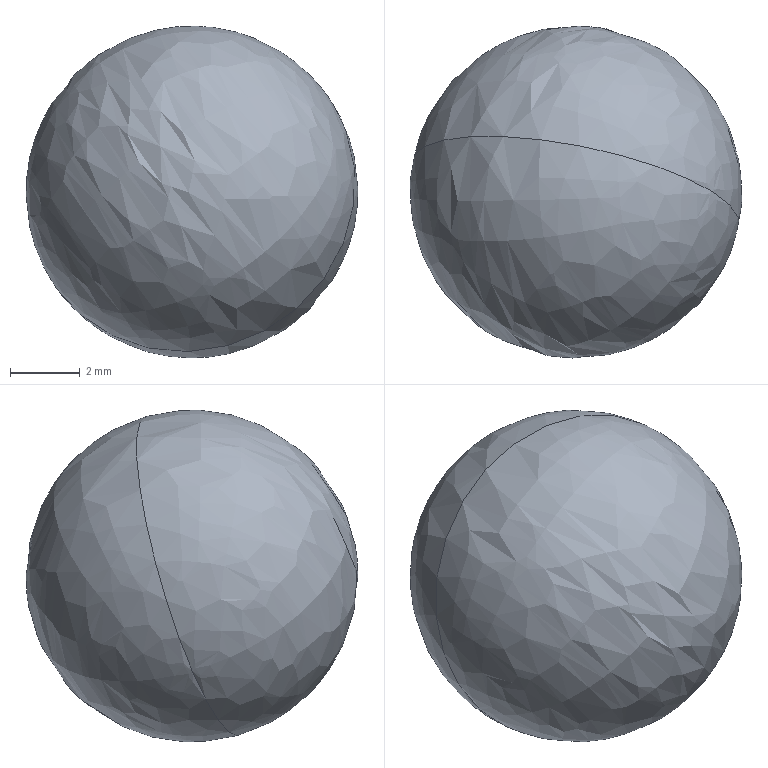Part | SolidWorks | features BaseBody 1 | 1 solid | 2 faces | box 9.525 x 9.525 x 9.525 mm | volume 452.463 mm3 | spline 2
STEP:
#1=CARTESIAN_POINT('',(3.904,63.008,68.627));
#2=VERTEX_POINT('',#1);
#3=CARTESIAN_POINT('',(-3.904,62.992,63.173));
#4=VERTEX_POINT('',#3);
#5=CARTESIAN_POINT('',(0.,63.,65.9));
#6=DIRECTION('',(-0.1902,-0.9425,0.2749));
#7=DIRECTION('',(0.8198,0.001585,0.5726));
#8=AXIS2_PLACEMENT_3D('',#5,#6,#7);
#9=CIRCLE('',#8,4.763);
#10=EDGE_CURVE('',#2,#4,#9,.T.);
#11=ORIENTED_EDGE('',*,*,#10,.F.);
#12=CARTESIAN_POINT('',(0.,63.,65.9));
#13=DIRECTION('',(0.1902,0.9425,-0.2749));
#14=DIRECTION('',(0.8198,0.001585,0.5726));
#15=AXIS2_PLACEMENT_3D('',#12,#13,#14);
#16=CIRCLE('',#15,4.763);
#17=EDGE_CURVE('',#2,#4,#16,.T.);
#18=ORIENTED_EDGE('',*,*,#17,.T.);
#19=EDGE_LOOP('',(#11,#18));
#20=FACE_OUTER_BOUND('',#19,.T.);
#21=CARTESIAN_POINT('',(3.904,63.008,68.627));
#22=CARTESIAN_POINT('',(3.904,63.008,68.627));
#23=CARTESIAN_POINT('',(3.904,63.008,68.627));
#24=CARTESIAN_POINT('',(3.904,63.008,68.627));
#25=CARTESIAN_POINT('',(9.049,59.823,61.271));
#26=CARTESIAN_POINT('',(12.673,77.777,56.033));
#27=CARTESIAN_POINT('',(2.384,84.146,70.746));
#28=CARTESIAN_POINT('',(-1.24,66.192,75.984));
#29=CARTESIAN_POINT('',(1.24,59.808,55.816));
#30=CARTESIAN_POINT('',(4.864,77.762,50.579));
#31=CARTESIAN_POINT('',(-5.425,84.131,65.291));
#32=CARTESIAN_POINT('',(-9.049,66.177,70.529));
#33=CARTESIAN_POINT('',(-3.904,62.992,63.173));
#34=CARTESIAN_POINT('',(-3.904,62.992,63.173));
#35=CARTESIAN_POINT('',(-3.904,62.992,63.173));
#36=CARTESIAN_POINT('',(-3.904,62.992,63.173));
#37=(BOUNDED_SURFACE()B_SPLINE_SURFACE(3,3,((#21,#22,#23,#24),(#25,#26,#27,#28),(#29,#30,#31,#32),(#33,#34,#35,#36)),.UNSPECIFIED.,.F.,.F.,.F.)B_SPLINE_SURFACE_WITH_KNOTS((4,4),(4,4),(0.,1.),(0.,1.),.UNSPECIFIED.)GEOMETRIC_REPRESENTATION_ITEM()RATIONAL_B_SPLINE_SURFACE(((1.,0.3333,0.3333,1.),(0.3333,0.1111,0.1111,0.3333),(0.3333,0.1111,0.1111,0.3333),(1.,0.3333,0.3333,1.)))REPRESENTATION_ITEM('')SURFACE());
#38=ADVANCED_FACE('',(#20),#37,.T.);
#39=ORIENTED_EDGE('',*,*,#17,.F.);
#40=ORIENTED_EDGE('',*,*,#10,.T.);
#41=EDGE_LOOP('',(#39,#40));
#42=FACE_OUTER_BOUND('',#41,.T.);
#43=CARTESIAN_POINT('',(3.904,63.008,68.627));
#44=CARTESIAN_POINT('',(3.904,63.008,68.627));
#45=CARTESIAN_POINT('',(3.904,63.008,68.627));
#46=CARTESIAN_POINT('',(3.904,63.008,68.627));
#47=CARTESIAN_POINT('',(-1.24,66.192,75.984));
#48=CARTESIAN_POINT('',(-4.864,48.238,81.221));
#49=CARTESIAN_POINT('',(5.425,41.869,66.509));
#50=CARTESIAN_POINT('',(9.049,59.823,61.271));
#51=CARTESIAN_POINT('',(-9.049,66.177,70.529));
#52=CARTESIAN_POINT('',(-12.673,48.223,75.767));
#53=CARTESIAN_POINT('',(-2.384,41.854,61.054));
#54=CARTESIAN_POINT('',(1.24,59.808,55.816));
#55=CARTESIAN_POINT('',(-3.904,62.992,63.173));
#56=CARTESIAN_POINT('',(-3.904,62.992,63.173));
#57=CARTESIAN_POINT('',(-3.904,62.992,63.173));
#58=CARTESIAN_POINT('',(-3.904,62.992,63.173));
#59=(BOUNDED_SURFACE()B_SPLINE_SURFACE(3,3,((#43,#44,#45,#46),(#47,#48,#49,#50),(#51,#52,#53,#54),(#55,#56,#57,#58)),.UNSPECIFIED.,.F.,.F.,.F.)B_SPLINE_SURFACE_WITH_KNOTS((4,4),(4,4),(0.,1.),(0.,1.),.UNSPECIFIED.)GEOMETRIC_REPRESENTATION_ITEM()RATIONAL_B_SPLINE_SURFACE(((1.,0.3333,0.3333,1.),(0.3333,0.1111,0.1111,0.3333),(0.3333,0.1111,0.1111,0.3333),(1.,0.3333,0.3333,1.)))REPRESENTATION_ITEM('')SURFACE());
#60=ADVANCED_FACE('',(#42),#59,.T.);
#61=CLOSED_SHELL('',(#38,#60));
#62=MANIFOLD_SOLID_BREP('',#61);
#63=CARTESIAN_POINT('',(0.,0.,0.));
#64=DIRECTION('',(0.,0.,1.));
#65=DIRECTION('',(1.,0.,0.));
#66=AXIS2_PLACEMENT_3D('',#63,#64,#65);
#67=(LENGTH_UNIT()NAMED_UNIT(*)SI_UNIT(.MILLI.,.METRE.));
#68=UNCERTAINTY_MEASURE_WITH_UNIT(LENGTH_MEASURE(0.00001),#67,'','');
#69=(NAMED_UNIT(*)PLANE_ANGLE_UNIT()SI_UNIT($,.RADIAN.));
#70=(NAMED_UNIT(*)SI_UNIT($,.STERADIAN.)SOLID_ANGLE_UNIT());
#71=(GEOMETRIC_REPRESENTATION_CONTEXT(3)GLOBAL_UNCERTAINTY_ASSIGNED_CONTEXT((#68))GLOBAL_UNIT_ASSIGNED_CONTEXT((#67,#69,#70))REPRESENTATION_CONTEXT('',''));
#72=ADVANCED_BREP_SHAPE_REPRESENTATION('',(#62,#66),#71);